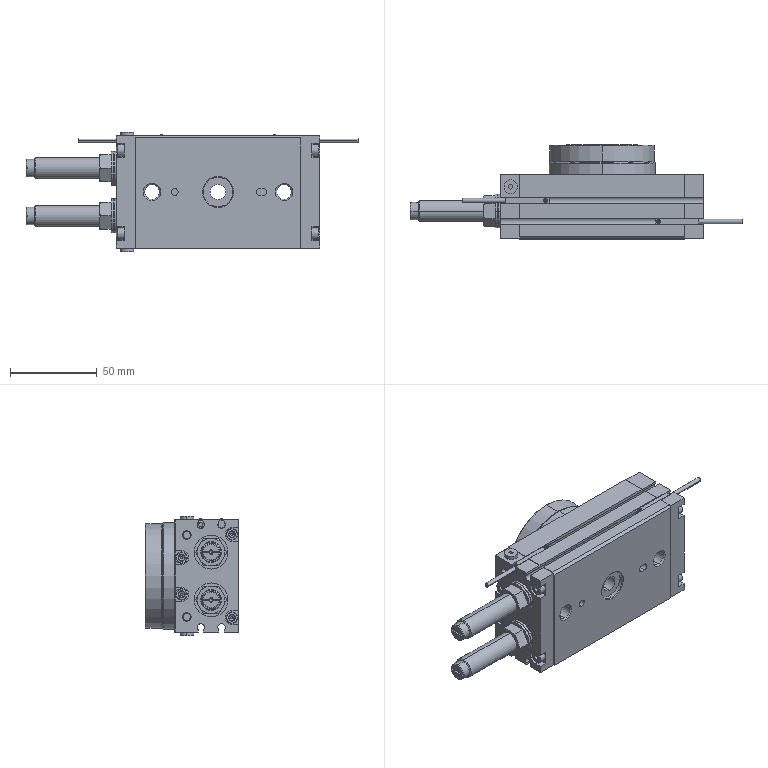Part | SolidWorks | 3 solids | 582 faces | box 191 x 54 x 69 mm | volume 317476 mm3 | plane 212 | cylinder 184 | cone 158 | torus 28 | commonest cylinder face diameters 6.66 x28 4.917 x24 4 x18 3.5 x16 2.572 x12 6.16 x12